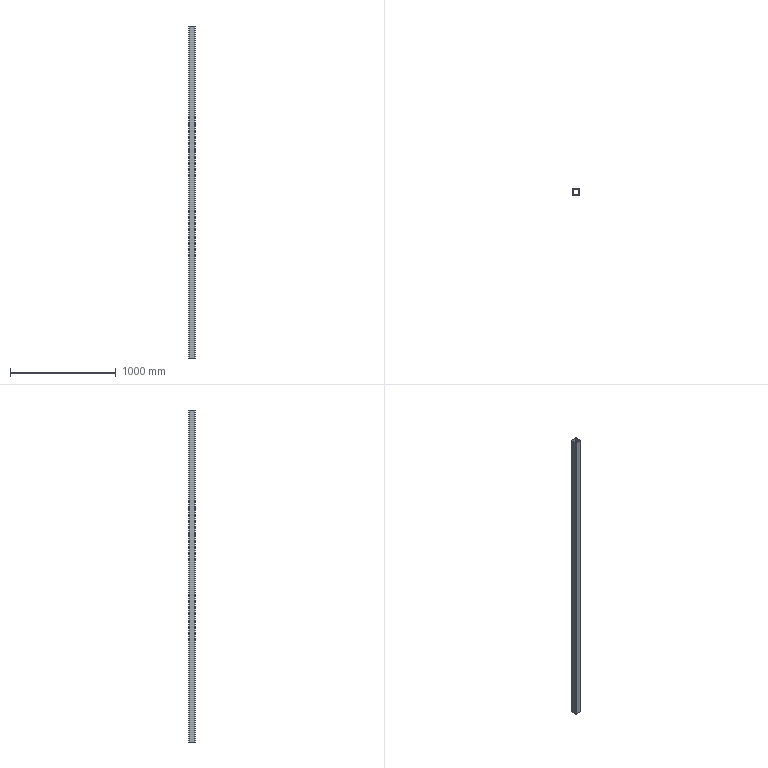Part | STEP file | X77-03101 | 1 solid | 14 faces | box 60 x 60 x 3140 mm | volume 2123501 mm3 | plane 10 | cylinder 4 | commonest cylinder face diameters 6 x4
STEP:
#1=CARTESIAN_POINT('',(0.,3.,3140.));
#2=VERTEX_POINT('',#1);
#3=CARTESIAN_POINT('',(3.,0.,3140.));
#4=VERTEX_POINT('',#3);
#5=CARTESIAN_POINT('',(3.,3.,3140.));
#6=DIRECTION('',(0.,0.,1.));
#7=DIRECTION('',(1.,0.,0.));
#8=AXIS2_PLACEMENT_3D('',#5,#6,#7);
#9=CIRCLE('',#8,3.);
#10=EDGE_CURVE('',#2,#4,#9,.T.);
#11=ORIENTED_EDGE('',*,*,#10,.T.);
#12=CARTESIAN_POINT('',(57.,0.,3140.));
#13=VERTEX_POINT('',#12);
#14=CARTESIAN_POINT('',(3.,0.,3140.));
#15=DIRECTION('',(1.,0.,0.));
#16=VECTOR('',#15,1000.);
#17=LINE('',#14,#16);
#18=EDGE_CURVE('',#4,#13,#17,.T.);
#19=ORIENTED_EDGE('',*,*,#18,.T.);
#20=CARTESIAN_POINT('',(60.,3.,3140.));
#21=VERTEX_POINT('',#20);
#22=CARTESIAN_POINT('',(57.,3.,3140.));
#23=DIRECTION('',(0.,0.,1.));
#24=DIRECTION('',(1.,0.,0.));
#25=AXIS2_PLACEMENT_3D('',#22,#23,#24);
#26=CIRCLE('',#25,3.);
#27=EDGE_CURVE('',#13,#21,#26,.T.);
#28=ORIENTED_EDGE('',*,*,#27,.T.);
#29=CARTESIAN_POINT('',(60.,57.,3140.));
#30=VERTEX_POINT('',#29);
#31=CARTESIAN_POINT('',(60.,3.,3140.));
#32=DIRECTION('',(0.,1.,0.));
#33=VECTOR('',#32,1000.);
#34=LINE('',#31,#33);
#35=EDGE_CURVE('',#21,#30,#34,.T.);
#36=ORIENTED_EDGE('',*,*,#35,.T.);
#37=CARTESIAN_POINT('',(57.,60.,3140.));
#38=VERTEX_POINT('',#37);
#39=CARTESIAN_POINT('',(57.,57.,3140.));
#40=DIRECTION('',(0.,0.,1.));
#41=DIRECTION('',(1.,0.,0.));
#42=AXIS2_PLACEMENT_3D('',#39,#40,#41);
#43=CIRCLE('',#42,3.);
#44=EDGE_CURVE('',#30,#38,#43,.T.);
#45=ORIENTED_EDGE('',*,*,#44,.T.);
#46=CARTESIAN_POINT('',(3.,60.,3140.));
#47=VERTEX_POINT('',#46);
#48=CARTESIAN_POINT('',(3.,60.,3140.));
#49=DIRECTION('',(-1.,0.,0.));
#50=VECTOR('',#49,1000.);
#51=LINE('',#48,#50);
#52=EDGE_CURVE('',#38,#47,#51,.T.);
#53=ORIENTED_EDGE('',*,*,#52,.T.);
#54=CARTESIAN_POINT('',(0.,57.,3140.));
#55=VERTEX_POINT('',#54);
#56=CARTESIAN_POINT('',(3.,57.,3140.));
#57=DIRECTION('',(0.,0.,1.));
#58=DIRECTION('',(1.,0.,0.));
#59=AXIS2_PLACEMENT_3D('',#56,#57,#58);
#60=CIRCLE('',#59,3.);
#61=EDGE_CURVE('',#47,#55,#60,.T.);
#62=ORIENTED_EDGE('',*,*,#61,.T.);
#63=CARTESIAN_POINT('',(0.,3.,3140.));
#64=DIRECTION('',(0.,-1.,0.));
#65=VECTOR('',#64,1000.);
#66=LINE('',#63,#65);
#67=EDGE_CURVE('',#55,#2,#66,.T.);
#68=ORIENTED_EDGE('',*,*,#67,.T.);
#69=EDGE_LOOP('',(#11,#19,#28,#36,#45,#53,#62,#68));
#70=FACE_OUTER_BOUND('',#69,.T.);
#71=CARTESIAN_POINT('',(3.,3.,3140.));
#72=VERTEX_POINT('',#71);
#73=CARTESIAN_POINT('',(57.,3.,3140.));
#74=VERTEX_POINT('',#73);
#75=CARTESIAN_POINT('',(3.,3.,3140.));
#76=DIRECTION('',(1.,0.,0.));
#77=VECTOR('',#76,1000.);
#78=LINE('',#75,#77);
#79=EDGE_CURVE('',#72,#74,#78,.T.);
#80=ORIENTED_EDGE('',*,*,#79,.F.);
#81=CARTESIAN_POINT('',(3.,57.,3140.));
#82=VERTEX_POINT('',#81);
#83=CARTESIAN_POINT('',(3.,3.,3140.));
#84=DIRECTION('',(0.,-1.,0.));
#85=VECTOR('',#84,1000.);
#86=LINE('',#83,#85);
#87=EDGE_CURVE('',#82,#72,#86,.T.);
#88=ORIENTED_EDGE('',*,*,#87,.F.);
#89=CARTESIAN_POINT('',(57.,57.,3140.));
#90=VERTEX_POINT('',#89);
#91=CARTESIAN_POINT('',(3.,57.,3140.));
#92=DIRECTION('',(-1.,0.,0.));
#93=VECTOR('',#92,1000.);
#94=LINE('',#91,#93);
#95=EDGE_CURVE('',#90,#82,#94,.T.);
#96=ORIENTED_EDGE('',*,*,#95,.F.);
#97=CARTESIAN_POINT('',(57.,3.,3140.));
#98=DIRECTION('',(0.,1.,0.));
#99=VECTOR('',#98,1000.);
#100=LINE('',#97,#99);
#101=EDGE_CURVE('',#74,#90,#100,.T.);
#102=ORIENTED_EDGE('',*,*,#101,.F.);
#103=EDGE_LOOP('',(#80,#88,#96,#102));
#104=FACE_BOUND('',#103,.T.);
#105=CARTESIAN_POINT('',(3.,3.,3140.));
#106=DIRECTION('',(0.,0.,1.));
#107=DIRECTION('',(1.,0.,0.));
#108=AXIS2_PLACEMENT_3D('',#105,#106,#107);
#109=PLANE('',#108);
#110=ADVANCED_FACE('',(#70,#104),#109,.T.);
#111=CARTESIAN_POINT('',(0.,3.,0.));
#112=VERTEX_POINT('',#111);
#113=CARTESIAN_POINT('',(3.,0.,0.));
#114=VERTEX_POINT('',#113);
#115=CARTESIAN_POINT('',(3.,3.,0.));
#116=DIRECTION('',(0.,0.,1.));
#117=DIRECTION('',(1.,0.,0.));
#118=AXIS2_PLACEMENT_3D('',#115,#116,#117);
#119=CIRCLE('',#118,3.);
#120=EDGE_CURVE('',#112,#114,#119,.T.);
#121=ORIENTED_EDGE('',*,*,#120,.F.);
#122=CARTESIAN_POINT('',(0.,57.,0.));
#123=VERTEX_POINT('',#122);
#124=CARTESIAN_POINT('',(0.,3.,0.));
#125=DIRECTION('',(0.,-1.,0.));
#126=VECTOR('',#125,1000.);
#127=LINE('',#124,#126);
#128=EDGE_CURVE('',#123,#112,#127,.T.);
#129=ORIENTED_EDGE('',*,*,#128,.F.);
#130=CARTESIAN_POINT('',(3.,60.,0.));
#131=VERTEX_POINT('',#130);
#132=CARTESIAN_POINT('',(3.,57.,0.));
#133=DIRECTION('',(0.,0.,1.));
#134=DIRECTION('',(1.,0.,0.));
#135=AXIS2_PLACEMENT_3D('',#132,#133,#134);
#136=CIRCLE('',#135,3.);
#137=EDGE_CURVE('',#131,#123,#136,.T.);
#138=ORIENTED_EDGE('',*,*,#137,.F.);
#139=CARTESIAN_POINT('',(57.,60.,0.));
#140=VERTEX_POINT('',#139);
#141=CARTESIAN_POINT('',(3.,60.,0.));
#142=DIRECTION('',(-1.,0.,0.));
#143=VECTOR('',#142,1000.);
#144=LINE('',#141,#143);
#145=EDGE_CURVE('',#140,#131,#144,.T.);
#146=ORIENTED_EDGE('',*,*,#145,.F.);
#147=CARTESIAN_POINT('',(60.,57.,0.));
#148=VERTEX_POINT('',#147);
#149=CARTESIAN_POINT('',(57.,57.,0.));
#150=DIRECTION('',(0.,0.,1.));
#151=DIRECTION('',(1.,0.,0.));
#152=AXIS2_PLACEMENT_3D('',#149,#150,#151);
#153=CIRCLE('',#152,3.);
#154=EDGE_CURVE('',#148,#140,#153,.T.);
#155=ORIENTED_EDGE('',*,*,#154,.F.);
#156=CARTESIAN_POINT('',(60.,3.,0.));
#157=VERTEX_POINT('',#156);
#158=CARTESIAN_POINT('',(60.,3.,0.));
#159=DIRECTION('',(0.,1.,0.));
#160=VECTOR('',#159,1000.);
#161=LINE('',#158,#160);
#162=EDGE_CURVE('',#157,#148,#161,.T.);
#163=ORIENTED_EDGE('',*,*,#162,.F.);
#164=CARTESIAN_POINT('',(57.,0.,0.));
#165=VERTEX_POINT('',#164);
#166=CARTESIAN_POINT('',(57.,3.,0.));
#167=DIRECTION('',(0.,0.,1.));
#168=DIRECTION('',(1.,0.,0.));
#169=AXIS2_PLACEMENT_3D('',#166,#167,#168);
#170=CIRCLE('',#169,3.);
#171=EDGE_CURVE('',#165,#157,#170,.T.);
#172=ORIENTED_EDGE('',*,*,#171,.F.);
#173=CARTESIAN_POINT('',(3.,0.,0.));
#174=DIRECTION('',(1.,0.,0.));
#175=VECTOR('',#174,1000.);
#176=LINE('',#173,#175);
#177=EDGE_CURVE('',#114,#165,#176,.T.);
#178=ORIENTED_EDGE('',*,*,#177,.F.);
#179=EDGE_LOOP('',(#121,#129,#138,#146,#155,#163,#172,#178));
#180=FACE_OUTER_BOUND('',#179,.T.);
#181=CARTESIAN_POINT('',(3.,57.,0.));
#182=VERTEX_POINT('',#181);
#183=CARTESIAN_POINT('',(3.,3.,0.));
#184=VERTEX_POINT('',#183);
#185=CARTESIAN_POINT('',(3.,3.,0.));
#186=DIRECTION('',(0.,-1.,0.));
#187=VECTOR('',#186,1000.);
#188=LINE('',#185,#187);
#189=EDGE_CURVE('',#182,#184,#188,.T.);
#190=ORIENTED_EDGE('',*,*,#189,.T.);
#191=CARTESIAN_POINT('',(57.,3.,0.));
#192=VERTEX_POINT('',#191);
#193=CARTESIAN_POINT('',(3.,3.,0.));
#194=DIRECTION('',(1.,0.,0.));
#195=VECTOR('',#194,1000.);
#196=LINE('',#193,#195);
#197=EDGE_CURVE('',#184,#192,#196,.T.);
#198=ORIENTED_EDGE('',*,*,#197,.T.);
#199=CARTESIAN_POINT('',(57.,57.,0.));
#200=VERTEX_POINT('',#199);
#201=CARTESIAN_POINT('',(57.,3.,0.));
#202=DIRECTION('',(0.,1.,0.));
#203=VECTOR('',#202,1000.);
#204=LINE('',#201,#203);
#205=EDGE_CURVE('',#192,#200,#204,.T.);
#206=ORIENTED_EDGE('',*,*,#205,.T.);
#207=CARTESIAN_POINT('',(3.,57.,0.));
#208=DIRECTION('',(-1.,0.,0.));
#209=VECTOR('',#208,1000.);
#210=LINE('',#207,#209);
#211=EDGE_CURVE('',#200,#182,#210,.T.);
#212=ORIENTED_EDGE('',*,*,#211,.T.);
#213=EDGE_LOOP('',(#190,#198,#206,#212));
#214=FACE_BOUND('',#213,.T.);
#215=CARTESIAN_POINT('',(3.,3.,0.));
#216=DIRECTION('',(0.,0.,1.));
#217=DIRECTION('',(1.,0.,0.));
#218=AXIS2_PLACEMENT_3D('',#215,#216,#217);
#219=PLANE('',#218);
#220=ADVANCED_FACE('',(#180,#214),#219,.F.);
#221=ORIENTED_EDGE('',*,*,#120,.T.);
#222=CARTESIAN_POINT('',(3.,0.,3140.));
#223=DIRECTION('',(0.,0.,-1.));
#224=VECTOR('',#223,1000.);
#225=LINE('',#222,#224);
#226=EDGE_CURVE('',#4,#114,#225,.T.);
#227=ORIENTED_EDGE('',*,*,#226,.F.);
#228=ORIENTED_EDGE('',*,*,#10,.F.);
#229=CARTESIAN_POINT('',(0.,3.,3140.));
#230=DIRECTION('',(0.,0.,-1.));
#231=VECTOR('',#230,1000.);
#232=LINE('',#229,#231);
#233=EDGE_CURVE('',#2,#112,#232,.T.);
#234=ORIENTED_EDGE('',*,*,#233,.T.);
#235=EDGE_LOOP('',(#221,#227,#228,#234));
#236=FACE_OUTER_BOUND('',#235,.T.);
#237=CARTESIAN_POINT('',(3.,3.,3140.));
#238=DIRECTION('',(0.,0.,-1.));
#239=DIRECTION('',(-1.,0.,0.));
#240=AXIS2_PLACEMENT_3D('',#237,#238,#239);
#241=CYLINDRICAL_SURFACE('',#240,3.);
#242=ADVANCED_FACE('',(#236),#241,.T.);
#243=ORIENTED_EDGE('',*,*,#177,.T.);
#244=CARTESIAN_POINT('',(57.,0.,3140.));
#245=DIRECTION('',(0.,0.,-1.));
#246=VECTOR('',#245,1000.);
#247=LINE('',#244,#246);
#248=EDGE_CURVE('',#13,#165,#247,.T.);
#249=ORIENTED_EDGE('',*,*,#248,.F.);
#250=ORIENTED_EDGE('',*,*,#18,.F.);
#251=ORIENTED_EDGE('',*,*,#226,.T.);
#252=EDGE_LOOP('',(#243,#249,#250,#251));
#253=FACE_OUTER_BOUND('',#252,.T.);
#254=CARTESIAN_POINT('',(3.,0.,3140.));
#255=DIRECTION('',(0.,1.,0.));
#256=DIRECTION('',(0.,0.,1.));
#257=AXIS2_PLACEMENT_3D('',#254,#255,#256);
#258=PLANE('',#257);
#259=ADVANCED_FACE('',(#253),#258,.F.);
#260=ORIENTED_EDGE('',*,*,#171,.T.);
#261=CARTESIAN_POINT('',(60.,3.,3140.));
#262=DIRECTION('',(0.,0.,-1.));
#263=VECTOR('',#262,1000.);
#264=LINE('',#261,#263);
#265=EDGE_CURVE('',#21,#157,#264,.T.);
#266=ORIENTED_EDGE('',*,*,#265,.F.);
#267=ORIENTED_EDGE('',*,*,#27,.F.);
#268=ORIENTED_EDGE('',*,*,#248,.T.);
#269=EDGE_LOOP('',(#260,#266,#267,#268));
#270=FACE_OUTER_BOUND('',#269,.T.);
#271=CARTESIAN_POINT('',(57.,3.,3140.));
#272=DIRECTION('',(0.,0.,-1.));
#273=DIRECTION('',(-1.,0.,0.));
#274=AXIS2_PLACEMENT_3D('',#271,#272,#273);
#275=CYLINDRICAL_SURFACE('',#274,3.);
#276=ADVANCED_FACE('',(#270),#275,.T.);
#277=ORIENTED_EDGE('',*,*,#162,.T.);
#278=CARTESIAN_POINT('',(60.,57.,3140.));
#279=DIRECTION('',(0.,0.,-1.));
#280=VECTOR('',#279,1000.);
#281=LINE('',#278,#280);
#282=EDGE_CURVE('',#30,#148,#281,.T.);
#283=ORIENTED_EDGE('',*,*,#282,.F.);
#284=ORIENTED_EDGE('',*,*,#35,.F.);
#285=ORIENTED_EDGE('',*,*,#265,.T.);
#286=EDGE_LOOP('',(#277,#283,#284,#285));
#287=FACE_OUTER_BOUND('',#286,.T.);
#288=CARTESIAN_POINT('',(60.,3.,3140.));
#289=DIRECTION('',(-1.,0.,0.));
#290=DIRECTION('',(0.,0.,1.));
#291=AXIS2_PLACEMENT_3D('',#288,#289,#290);
#292=PLANE('',#291);
#293=ADVANCED_FACE('',(#287),#292,.F.);
#294=ORIENTED_EDGE('',*,*,#154,.T.);
#295=CARTESIAN_POINT('',(57.,60.,3140.));
#296=DIRECTION('',(0.,0.,-1.));
#297=VECTOR('',#296,1000.);
#298=LINE('',#295,#297);
#299=EDGE_CURVE('',#38,#140,#298,.T.);
#300=ORIENTED_EDGE('',*,*,#299,.F.);
#301=ORIENTED_EDGE('',*,*,#44,.F.);
#302=ORIENTED_EDGE('',*,*,#282,.T.);
#303=EDGE_LOOP('',(#294,#300,#301,#302));
#304=FACE_OUTER_BOUND('',#303,.T.);
#305=CARTESIAN_POINT('',(57.,57.,3140.));
#306=DIRECTION('',(0.,0.,-1.));
#307=DIRECTION('',(-1.,0.,0.));
#308=AXIS2_PLACEMENT_3D('',#305,#306,#307);
#309=CYLINDRICAL_SURFACE('',#308,3.);
#310=ADVANCED_FACE('',(#304),#309,.T.);
#311=ORIENTED_EDGE('',*,*,#145,.T.);
#312=CARTESIAN_POINT('',(3.,60.,3140.));
#313=DIRECTION('',(0.,0.,-1.));
#314=VECTOR('',#313,1000.);
#315=LINE('',#312,#314);
#316=EDGE_CURVE('',#47,#131,#315,.T.);
#317=ORIENTED_EDGE('',*,*,#316,.F.);
#318=ORIENTED_EDGE('',*,*,#52,.F.);
#319=ORIENTED_EDGE('',*,*,#299,.T.);
#320=EDGE_LOOP('',(#311,#317,#318,#319));
#321=FACE_OUTER_BOUND('',#320,.T.);
#322=CARTESIAN_POINT('',(3.,60.,3140.));
#323=DIRECTION('',(0.,-1.,0.));
#324=DIRECTION('',(0.,0.,-1.));
#325=AXIS2_PLACEMENT_3D('',#322,#323,#324);
#326=PLANE('',#325);
#327=ADVANCED_FACE('',(#321),#326,.F.);
#328=ORIENTED_EDGE('',*,*,#137,.T.);
#329=CARTESIAN_POINT('',(0.,57.,3140.));
#330=DIRECTION('',(0.,0.,-1.));
#331=VECTOR('',#330,1000.);
#332=LINE('',#329,#331);
#333=EDGE_CURVE('',#55,#123,#332,.T.);
#334=ORIENTED_EDGE('',*,*,#333,.F.);
#335=ORIENTED_EDGE('',*,*,#61,.F.);
#336=ORIENTED_EDGE('',*,*,#316,.T.);
#337=EDGE_LOOP('',(#328,#334,#335,#336));
#338=FACE_OUTER_BOUND('',#337,.T.);
#339=CARTESIAN_POINT('',(3.,57.,3140.));
#340=DIRECTION('',(0.,0.,-1.));
#341=DIRECTION('',(-1.,0.,0.));
#342=AXIS2_PLACEMENT_3D('',#339,#340,#341);
#343=CYLINDRICAL_SURFACE('',#342,3.);
#344=ADVANCED_FACE('',(#338),#343,.T.);
#345=ORIENTED_EDGE('',*,*,#128,.T.);
#346=ORIENTED_EDGE('',*,*,#233,.F.);
#347=ORIENTED_EDGE('',*,*,#67,.F.);
#348=ORIENTED_EDGE('',*,*,#333,.T.);
#349=EDGE_LOOP('',(#345,#346,#347,#348));
#350=FACE_OUTER_BOUND('',#349,.T.);
#351=CARTESIAN_POINT('',(0.,3.,3140.));
#352=DIRECTION('',(1.,0.,0.));
#353=DIRECTION('',(0.,0.,-1.));
#354=AXIS2_PLACEMENT_3D('',#351,#352,#353);
#355=PLANE('',#354);
#356=ADVANCED_FACE('',(#350),#355,.F.);
#357=ORIENTED_EDGE('',*,*,#189,.F.);
#358=CARTESIAN_POINT('',(3.,57.,3140.));
#359=DIRECTION('',(0.,0.,-1.));
#360=VECTOR('',#359,1000.);
#361=LINE('',#358,#360);
#362=EDGE_CURVE('',#82,#182,#361,.T.);
#363=ORIENTED_EDGE('',*,*,#362,.F.);
#364=ORIENTED_EDGE('',*,*,#87,.T.);
#365=CARTESIAN_POINT('',(3.,3.,3140.));
#366=DIRECTION('',(0.,0.,-1.));
#367=VECTOR('',#366,1000.);
#368=LINE('',#365,#367);
#369=EDGE_CURVE('',#72,#184,#368,.T.);
#370=ORIENTED_EDGE('',*,*,#369,.T.);
#371=EDGE_LOOP('',(#357,#363,#364,#370));
#372=FACE_OUTER_BOUND('',#371,.T.);
#373=CARTESIAN_POINT('',(3.,3.,3140.));
#374=DIRECTION('',(1.,0.,0.));
#375=DIRECTION('',(0.,0.,-1.));
#376=AXIS2_PLACEMENT_3D('',#373,#374,#375);
#377=PLANE('',#376);
#378=ADVANCED_FACE('',(#372),#377,.T.);
#379=ORIENTED_EDGE('',*,*,#197,.F.);
#380=ORIENTED_EDGE('',*,*,#369,.F.);
#381=ORIENTED_EDGE('',*,*,#79,.T.);
#382=CARTESIAN_POINT('',(57.,3.,3140.));
#383=DIRECTION('',(0.,0.,-1.));
#384=VECTOR('',#383,1000.);
#385=LINE('',#382,#384);
#386=EDGE_CURVE('',#74,#192,#385,.T.);
#387=ORIENTED_EDGE('',*,*,#386,.T.);
#388=EDGE_LOOP('',(#379,#380,#381,#387));
#389=FACE_OUTER_BOUND('',#388,.T.);
#390=CARTESIAN_POINT('',(3.,3.,3140.));
#391=DIRECTION('',(0.,1.,0.));
#392=DIRECTION('',(0.,0.,1.));
#393=AXIS2_PLACEMENT_3D('',#390,#391,#392);
#394=PLANE('',#393);
#395=ADVANCED_FACE('',(#389),#394,.T.);
#396=ORIENTED_EDGE('',*,*,#205,.F.);
#397=ORIENTED_EDGE('',*,*,#386,.F.);
#398=ORIENTED_EDGE('',*,*,#101,.T.);
#399=CARTESIAN_POINT('',(57.,57.,3140.));
#400=DIRECTION('',(0.,0.,-1.));
#401=VECTOR('',#400,1000.);
#402=LINE('',#399,#401);
#403=EDGE_CURVE('',#90,#200,#402,.T.);
#404=ORIENTED_EDGE('',*,*,#403,.T.);
#405=EDGE_LOOP('',(#396,#397,#398,#404));
#406=FACE_OUTER_BOUND('',#405,.T.);
#407=CARTESIAN_POINT('',(57.,3.,3140.));
#408=DIRECTION('',(-1.,0.,0.));
#409=DIRECTION('',(0.,0.,1.));
#410=AXIS2_PLACEMENT_3D('',#407,#408,#409);
#411=PLANE('',#410);
#412=ADVANCED_FACE('',(#406),#411,.T.);
#413=ORIENTED_EDGE('',*,*,#211,.F.);
#414=ORIENTED_EDGE('',*,*,#403,.F.);
#415=ORIENTED_EDGE('',*,*,#95,.T.);
#416=ORIENTED_EDGE('',*,*,#362,.T.);
#417=EDGE_LOOP('',(#413,#414,#415,#416));
#418=FACE_OUTER_BOUND('',#417,.T.);
#419=CARTESIAN_POINT('',(3.,57.,3140.));
#420=DIRECTION('',(0.,-1.,0.));
#421=DIRECTION('',(0.,0.,-1.));
#422=AXIS2_PLACEMENT_3D('',#419,#420,#421);
#423=PLANE('',#422);
#424=ADVANCED_FACE('',(#418),#423,.T.);
#425=CLOSED_SHELL('',(#110,#220,#242,#259,#276,#293,#310,#327,#344,#356,#378,#395,#412,#424));
#426=MANIFOLD_SOLID_BREP('',#425);
#427=CARTESIAN_POINT('',(0.,0.,0.));
#428=DIRECTION('',(0.,0.,1.));
#429=DIRECTION('',(1.,0.,0.));
#430=AXIS2_PLACEMENT_3D('',#427,#428,#429);
#431=(LENGTH_UNIT()NAMED_UNIT(*)SI_UNIT(.MILLI.,.METRE.));
#432=UNCERTAINTY_MEASURE_WITH_UNIT(LENGTH_MEASURE(0.00001),#431,'','');
#433=(NAMED_UNIT(*)PLANE_ANGLE_UNIT()SI_UNIT($,.RADIAN.));
#434=(NAMED_UNIT(*)SI_UNIT($,.STERADIAN.)SOLID_ANGLE_UNIT());
#435=(GEOMETRIC_REPRESENTATION_CONTEXT(3)GLOBAL_UNCERTAINTY_ASSIGNED_CONTEXT((#432))GLOBAL_UNIT_ASSIGNED_CONTEXT((#431,#433,#434))REPRESENTATION_CONTEXT('',''));
#436=ADVANCED_BREP_SHAPE_REPRESENTATION('',(#426,#430),#435);